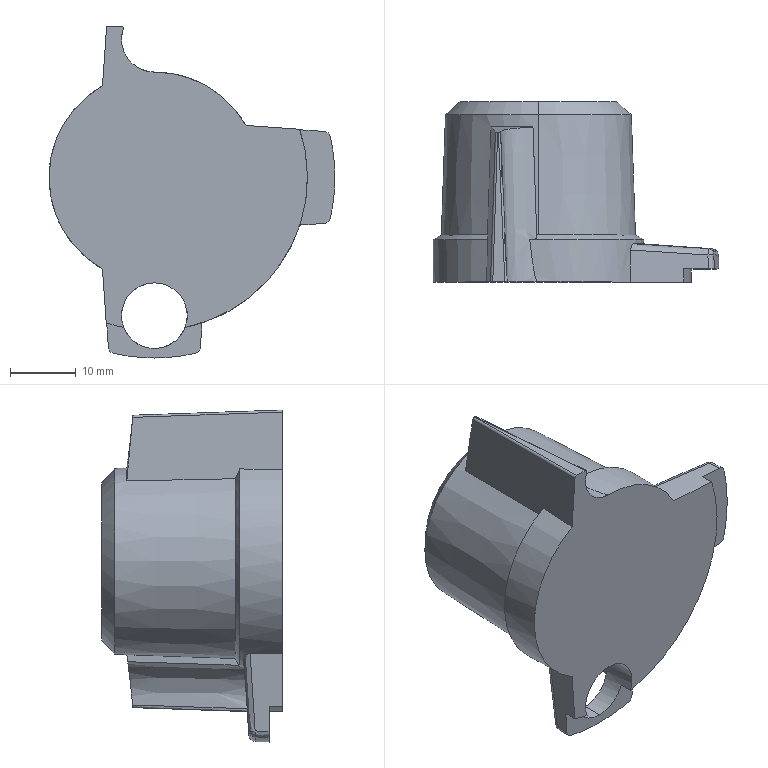Part | STEP file | VHS30-03_VHS3035BA Handle_30 | 1 solid | 58 faces | box 43.43 x 27.4 x 50.43 mm | volume 21299 mm3 | cone 18 | plane 14 | spline 10 | cylinder 9 | sphere 4 | torus 3 | commonest cylinder face diameters 32 x3 0.7 x2 10 x2 46.5 x2